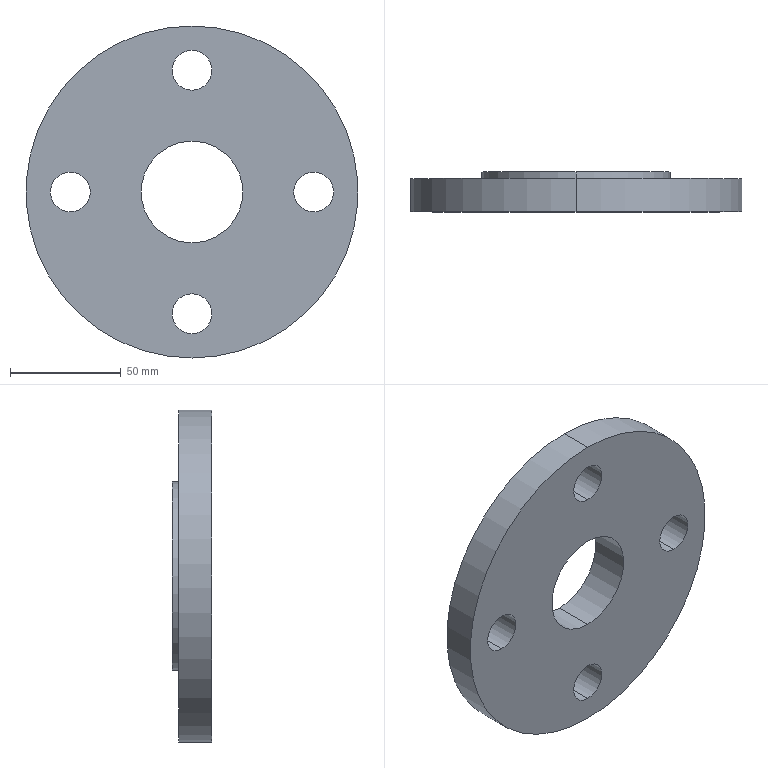Part | SolidWorks | features Extrusion 1, ICE 1 | 1 solid | 17 faces | box 150 x 18 x 150 mm | volume 236913 mm3 | cylinder 14 | plane 3 | commonest cylinder face diameters 18 x8 46 x2 85 x2 150 x2
STEP:
#1=CARTESIAN_POINT('',(0.,18.,42.5));
#2=VERTEX_POINT('',#1);
#3=CARTESIAN_POINT('',(0.,18.,-42.5));
#4=VERTEX_POINT('',#3);
#5=CARTESIAN_POINT('',(0.,18.,0.));
#6=DIRECTION('',(0.,1.,0.));
#7=DIRECTION('',(0.,0.,1.));
#8=AXIS2_PLACEMENT_3D('',#5,#6,#7);
#9=CIRCLE('',#8,42.5);
#10=EDGE_CURVE('',#2,#4,#9,.T.);
#11=ORIENTED_EDGE('',*,*,#10,.F.);
#12=CARTESIAN_POINT('',(0.,15.,42.5));
#13=VERTEX_POINT('',#12);
#14=CARTESIAN_POINT('',(0.,18.,42.5));
#15=DIRECTION('',(0.,-1.,0.));
#16=VECTOR('',#15,1000.);
#17=LINE('',#14,#16);
#18=EDGE_CURVE('',#2,#13,#17,.T.);
#19=ORIENTED_EDGE('',*,*,#18,.T.);
#20=CARTESIAN_POINT('',(0.,15.,-42.5));
#21=VERTEX_POINT('',#20);
#22=CARTESIAN_POINT('',(0.,15.,0.));
#23=DIRECTION('',(0.,1.,0.));
#24=DIRECTION('',(0.,0.,1.));
#25=AXIS2_PLACEMENT_3D('',#22,#23,#24);
#26=CIRCLE('',#25,42.5);
#27=EDGE_CURVE('',#13,#21,#26,.T.);
#28=ORIENTED_EDGE('',*,*,#27,.T.);
#29=CARTESIAN_POINT('',(0.,18.,-42.5));
#30=DIRECTION('',(0.,-1.,0.));
#31=VECTOR('',#30,1000.);
#32=LINE('',#29,#31);
#33=EDGE_CURVE('',#4,#21,#32,.T.);
#34=ORIENTED_EDGE('',*,*,#33,.F.);
#35=EDGE_LOOP('',(#11,#19,#28,#34));
#36=FACE_OUTER_BOUND('',#35,.T.);
#37=CARTESIAN_POINT('',(0.,18.,0.));
#38=DIRECTION('',(0.,-1.,0.));
#39=DIRECTION('',(0.,0.,-1.));
#40=AXIS2_PLACEMENT_3D('',#37,#38,#39);
#41=CYLINDRICAL_SURFACE('',#40,42.5);
#42=ADVANCED_FACE('',(#36),#41,.T.);
#43=CARTESIAN_POINT('',(-55.,15.,-9.));
#44=VERTEX_POINT('',#43);
#45=CARTESIAN_POINT('',(-55.,15.,9.));
#46=VERTEX_POINT('',#45);
#47=CARTESIAN_POINT('',(-55.,15.,0.));
#48=DIRECTION('',(0.,1.,0.));
#49=DIRECTION('',(0.,0.,1.));
#50=AXIS2_PLACEMENT_3D('',#47,#48,#49);
#51=CIRCLE('',#50,9.);
#52=EDGE_CURVE('',#44,#46,#51,.T.);
#53=ORIENTED_EDGE('',*,*,#52,.T.);
#54=CARTESIAN_POINT('',(-55.,0.,9.));
#55=VERTEX_POINT('',#54);
#56=CARTESIAN_POINT('',(-55.,15.,9.));
#57=DIRECTION('',(0.,-1.,0.));
#58=VECTOR('',#57,1000.);
#59=LINE('',#56,#58);
#60=EDGE_CURVE('',#46,#55,#59,.T.);
#61=ORIENTED_EDGE('',*,*,#60,.T.);
#62=CARTESIAN_POINT('',(-55.,0.,-9.));
#63=VERTEX_POINT('',#62);
#64=CARTESIAN_POINT('',(-55.,0.,0.));
#65=DIRECTION('',(0.,1.,0.));
#66=DIRECTION('',(0.,0.,1.));
#67=AXIS2_PLACEMENT_3D('',#64,#65,#66);
#68=CIRCLE('',#67,9.);
#69=EDGE_CURVE('',#63,#55,#68,.T.);
#70=ORIENTED_EDGE('',*,*,#69,.F.);
#71=CARTESIAN_POINT('',(-55.,15.,-9.));
#72=DIRECTION('',(0.,-1.,0.));
#73=VECTOR('',#72,1000.);
#74=LINE('',#71,#73);
#75=EDGE_CURVE('',#44,#63,#74,.T.);
#76=ORIENTED_EDGE('',*,*,#75,.F.);
#77=EDGE_LOOP('',(#53,#61,#70,#76));
#78=FACE_OUTER_BOUND('',#77,.T.);
#79=CARTESIAN_POINT('',(-55.,15.,0.));
#80=DIRECTION('',(0.,-1.,0.));
#81=DIRECTION('',(0.,0.,-1.));
#82=AXIS2_PLACEMENT_3D('',#79,#80,#81);
#83=CYLINDRICAL_SURFACE('',#82,9.);
#84=ADVANCED_FACE('',(#78),#83,.F.);
#85=CARTESIAN_POINT('',(0.,15.,46.));
#86=VERTEX_POINT('',#85);
#87=CARTESIAN_POINT('',(0.,15.,64.));
#88=VERTEX_POINT('',#87);
#89=CARTESIAN_POINT('',(0.,15.,55.));
#90=DIRECTION('',(0.,1.,0.));
#91=DIRECTION('',(0.,0.,1.));
#92=AXIS2_PLACEMENT_3D('',#89,#90,#91);
#93=CIRCLE('',#92,9.);
#94=EDGE_CURVE('',#86,#88,#93,.T.);
#95=ORIENTED_EDGE('',*,*,#94,.T.);
#96=CARTESIAN_POINT('',(0.,0.,64.));
#97=VERTEX_POINT('',#96);
#98=CARTESIAN_POINT('',(0.,15.,64.));
#99=DIRECTION('',(0.,-1.,0.));
#100=VECTOR('',#99,1000.);
#101=LINE('',#98,#100);
#102=EDGE_CURVE('',#88,#97,#101,.T.);
#103=ORIENTED_EDGE('',*,*,#102,.T.);
#104=CARTESIAN_POINT('',(0.,0.,46.));
#105=VERTEX_POINT('',#104);
#106=CARTESIAN_POINT('',(0.,0.,55.));
#107=DIRECTION('',(0.,1.,0.));
#108=DIRECTION('',(0.,0.,1.));
#109=AXIS2_PLACEMENT_3D('',#106,#107,#108);
#110=CIRCLE('',#109,9.);
#111=EDGE_CURVE('',#105,#97,#110,.T.);
#112=ORIENTED_EDGE('',*,*,#111,.F.);
#113=CARTESIAN_POINT('',(0.,15.,46.));
#114=DIRECTION('',(0.,-1.,0.));
#115=VECTOR('',#114,1000.);
#116=LINE('',#113,#115);
#117=EDGE_CURVE('',#86,#105,#116,.T.);
#118=ORIENTED_EDGE('',*,*,#117,.F.);
#119=EDGE_LOOP('',(#95,#103,#112,#118));
#120=FACE_OUTER_BOUND('',#119,.T.);
#121=CARTESIAN_POINT('',(0.,15.,55.));
#122=DIRECTION('',(0.,-1.,0.));
#123=DIRECTION('',(0.,0.,-1.));
#124=AXIS2_PLACEMENT_3D('',#121,#122,#123);
#125=CYLINDRICAL_SURFACE('',#124,9.);
#126=ADVANCED_FACE('',(#120),#125,.F.);
#127=CARTESIAN_POINT('',(55.,15.,-9.));
#128=VERTEX_POINT('',#127);
#129=CARTESIAN_POINT('',(55.,15.,9.));
#130=VERTEX_POINT('',#129);
#131=CARTESIAN_POINT('',(55.,15.,0.));
#132=DIRECTION('',(0.,1.,0.));
#133=DIRECTION('',(0.,0.,1.));
#134=AXIS2_PLACEMENT_3D('',#131,#132,#133);
#135=CIRCLE('',#134,9.);
#136=EDGE_CURVE('',#128,#130,#135,.T.);
#137=ORIENTED_EDGE('',*,*,#136,.T.);
#138=CARTESIAN_POINT('',(55.,0.,9.));
#139=VERTEX_POINT('',#138);
#140=CARTESIAN_POINT('',(55.,15.,9.));
#141=DIRECTION('',(0.,-1.,0.));
#142=VECTOR('',#141,1000.);
#143=LINE('',#140,#142);
#144=EDGE_CURVE('',#130,#139,#143,.T.);
#145=ORIENTED_EDGE('',*,*,#144,.T.);
#146=CARTESIAN_POINT('',(55.,0.,-9.));
#147=VERTEX_POINT('',#146);
#148=CARTESIAN_POINT('',(55.,0.,0.));
#149=DIRECTION('',(0.,1.,0.));
#150=DIRECTION('',(0.,0.,1.));
#151=AXIS2_PLACEMENT_3D('',#148,#149,#150);
#152=CIRCLE('',#151,9.);
#153=EDGE_CURVE('',#147,#139,#152,.T.);
#154=ORIENTED_EDGE('',*,*,#153,.F.);
#155=CARTESIAN_POINT('',(55.,15.,-9.));
#156=DIRECTION('',(0.,-1.,0.));
#157=VECTOR('',#156,1000.);
#158=LINE('',#155,#157);
#159=EDGE_CURVE('',#128,#147,#158,.T.);
#160=ORIENTED_EDGE('',*,*,#159,.F.);
#161=EDGE_LOOP('',(#137,#145,#154,#160));
#162=FACE_OUTER_BOUND('',#161,.T.);
#163=CARTESIAN_POINT('',(55.,15.,0.));
#164=DIRECTION('',(0.,-1.,0.));
#165=DIRECTION('',(0.,0.,-1.));
#166=AXIS2_PLACEMENT_3D('',#163,#164,#165);
#167=CYLINDRICAL_SURFACE('',#166,9.);
#168=ADVANCED_FACE('',(#162),#167,.F.);
#169=CARTESIAN_POINT('',(0.,18.,-23.));
#170=VERTEX_POINT('',#169);
#171=CARTESIAN_POINT('',(0.,18.,23.));
#172=VERTEX_POINT('',#171);
#173=CARTESIAN_POINT('',(0.,18.,0.));
#174=DIRECTION('',(0.,1.,0.));
#175=DIRECTION('',(0.,0.,1.));
#176=AXIS2_PLACEMENT_3D('',#173,#174,#175);
#177=CIRCLE('',#176,23.);
#178=EDGE_CURVE('',#170,#172,#177,.T.);
#179=ORIENTED_EDGE('',*,*,#178,.T.);
#180=CARTESIAN_POINT('',(0.,0.,23.));
#181=VERTEX_POINT('',#180);
#182=CARTESIAN_POINT('',(0.,15.,23.));
#183=DIRECTION('',(0.,-1.,0.));
#184=VECTOR('',#183,1000.);
#185=LINE('',#182,#184);
#186=EDGE_CURVE('',#172,#181,#185,.T.);
#187=ORIENTED_EDGE('',*,*,#186,.T.);
#188=CARTESIAN_POINT('',(0.,0.,-23.));
#189=VERTEX_POINT('',#188);
#190=CARTESIAN_POINT('',(0.,0.,0.));
#191=DIRECTION('',(0.,1.,0.));
#192=DIRECTION('',(0.,0.,1.));
#193=AXIS2_PLACEMENT_3D('',#190,#191,#192);
#194=CIRCLE('',#193,23.);
#195=EDGE_CURVE('',#189,#181,#194,.T.);
#196=ORIENTED_EDGE('',*,*,#195,.F.);
#197=CARTESIAN_POINT('',(0.,15.,-23.));
#198=DIRECTION('',(0.,-1.,0.));
#199=VECTOR('',#198,1000.);
#200=LINE('',#197,#199);
#201=EDGE_CURVE('',#170,#189,#200,.T.);
#202=ORIENTED_EDGE('',*,*,#201,.F.);
#203=EDGE_LOOP('',(#179,#187,#196,#202));
#204=FACE_OUTER_BOUND('',#203,.T.);
#205=CARTESIAN_POINT('',(0.,15.,0.));
#206=DIRECTION('',(0.,-1.,0.));
#207=DIRECTION('',(0.,0.,-1.));
#208=AXIS2_PLACEMENT_3D('',#205,#206,#207);
#209=CYLINDRICAL_SURFACE('',#208,23.);
#210=ADVANCED_FACE('',(#204),#209,.F.);
#211=CARTESIAN_POINT('',(0.,15.,-64.));
#212=VERTEX_POINT('',#211);
#213=CARTESIAN_POINT('',(0.,15.,-46.));
#214=VERTEX_POINT('',#213);
#215=CARTESIAN_POINT('',(0.,15.,-55.));
#216=DIRECTION('',(0.,1.,0.));
#217=DIRECTION('',(0.,0.,1.));
#218=AXIS2_PLACEMENT_3D('',#215,#216,#217);
#219=CIRCLE('',#218,9.);
#220=EDGE_CURVE('',#212,#214,#219,.T.);
#221=ORIENTED_EDGE('',*,*,#220,.T.);
#222=CARTESIAN_POINT('',(0.,0.,-46.));
#223=VERTEX_POINT('',#222);
#224=CARTESIAN_POINT('',(0.,15.,-46.));
#225=DIRECTION('',(0.,-1.,0.));
#226=VECTOR('',#225,1000.);
#227=LINE('',#224,#226);
#228=EDGE_CURVE('',#214,#223,#227,.T.);
#229=ORIENTED_EDGE('',*,*,#228,.T.);
#230=CARTESIAN_POINT('',(0.,0.,-64.));
#231=VERTEX_POINT('',#230);
#232=CARTESIAN_POINT('',(0.,0.,-55.));
#233=DIRECTION('',(0.,1.,0.));
#234=DIRECTION('',(0.,0.,1.));
#235=AXIS2_PLACEMENT_3D('',#232,#233,#234);
#236=CIRCLE('',#235,9.);
#237=EDGE_CURVE('',#231,#223,#236,.T.);
#238=ORIENTED_EDGE('',*,*,#237,.F.);
#239=CARTESIAN_POINT('',(0.,15.,-64.));
#240=DIRECTION('',(0.,-1.,0.));
#241=VECTOR('',#240,1000.);
#242=LINE('',#239,#241);
#243=EDGE_CURVE('',#212,#231,#242,.T.);
#244=ORIENTED_EDGE('',*,*,#243,.F.);
#245=EDGE_LOOP('',(#221,#229,#238,#244));
#246=FACE_OUTER_BOUND('',#245,.T.);
#247=CARTESIAN_POINT('',(0.,15.,-55.));
#248=DIRECTION('',(0.,-1.,0.));
#249=DIRECTION('',(0.,0.,-1.));
#250=AXIS2_PLACEMENT_3D('',#247,#248,#249);
#251=CYLINDRICAL_SURFACE('',#250,9.);
#252=ADVANCED_FACE('',(#246),#251,.F.);
#253=CARTESIAN_POINT('',(0.,15.,75.));
#254=VERTEX_POINT('',#253);
#255=CARTESIAN_POINT('',(0.,15.,-75.));
#256=VERTEX_POINT('',#255);
#257=CARTESIAN_POINT('',(0.,15.,0.));
#258=DIRECTION('',(0.,1.,0.));
#259=DIRECTION('',(0.,0.,1.));
#260=AXIS2_PLACEMENT_3D('',#257,#258,#259);
#261=CIRCLE('',#260,75.);
#262=EDGE_CURVE('',#254,#256,#261,.T.);
#263=ORIENTED_EDGE('',*,*,#262,.F.);
#264=CARTESIAN_POINT('',(0.,0.,75.));
#265=VERTEX_POINT('',#264);
#266=CARTESIAN_POINT('',(0.,15.,75.));
#267=DIRECTION('',(0.,-1.,0.));
#268=VECTOR('',#267,1000.);
#269=LINE('',#266,#268);
#270=EDGE_CURVE('',#254,#265,#269,.T.);
#271=ORIENTED_EDGE('',*,*,#270,.T.);
#272=CARTESIAN_POINT('',(0.,0.,-75.));
#273=VERTEX_POINT('',#272);
#274=CARTESIAN_POINT('',(0.,0.,0.));
#275=DIRECTION('',(0.,1.,0.));
#276=DIRECTION('',(0.,0.,1.));
#277=AXIS2_PLACEMENT_3D('',#274,#275,#276);
#278=CIRCLE('',#277,75.);
#279=EDGE_CURVE('',#265,#273,#278,.T.);
#280=ORIENTED_EDGE('',*,*,#279,.T.);
#281=CARTESIAN_POINT('',(0.,15.,-75.));
#282=DIRECTION('',(0.,-1.,0.));
#283=VECTOR('',#282,1000.);
#284=LINE('',#281,#283);
#285=EDGE_CURVE('',#256,#273,#284,.T.);
#286=ORIENTED_EDGE('',*,*,#285,.F.);
#287=EDGE_LOOP('',(#263,#271,#280,#286));
#288=FACE_OUTER_BOUND('',#287,.T.);
#289=CARTESIAN_POINT('',(0.,15.,0.));
#290=DIRECTION('',(0.,-1.,0.));
#291=DIRECTION('',(0.,0.,-1.));
#292=AXIS2_PLACEMENT_3D('',#289,#290,#291);
#293=CYLINDRICAL_SURFACE('',#292,75.);
#294=ADVANCED_FACE('',(#288),#293,.T.);
#295=CARTESIAN_POINT('',(0.,15.,0.));
#296=DIRECTION('',(0.,1.,0.));
#297=DIRECTION('',(0.,0.,1.));
#298=AXIS2_PLACEMENT_3D('',#295,#296,#297);
#299=CIRCLE('',#298,42.5);
#300=EDGE_CURVE('',#21,#13,#299,.T.);
#301=ORIENTED_EDGE('',*,*,#300,.F.);
#302=ORIENTED_EDGE('',*,*,#27,.F.);
#303=EDGE_LOOP('',(#301,#302));
#304=FACE_BOUND('',#303,.T.);
#305=ORIENTED_EDGE('',*,*,#94,.F.);
#306=CARTESIAN_POINT('',(0.,15.,55.));
#307=DIRECTION('',(0.,1.,0.));
#308=DIRECTION('',(0.,0.,1.));
#309=AXIS2_PLACEMENT_3D('',#306,#307,#308);
#310=CIRCLE('',#309,9.);
#311=EDGE_CURVE('',#88,#86,#310,.T.);
#312=ORIENTED_EDGE('',*,*,#311,.F.);
#313=EDGE_LOOP('',(#305,#312));
#314=FACE_BOUND('',#313,.T.);
#315=CARTESIAN_POINT('',(0.,15.,0.));
#316=DIRECTION('',(0.,1.,0.));
#317=DIRECTION('',(0.,0.,1.));
#318=AXIS2_PLACEMENT_3D('',#315,#316,#317);
#319=CIRCLE('',#318,75.);
#320=EDGE_CURVE('',#256,#254,#319,.T.);
#321=ORIENTED_EDGE('',*,*,#320,.T.);
#322=ORIENTED_EDGE('',*,*,#262,.T.);
#323=EDGE_LOOP('',(#321,#322));
#324=FACE_OUTER_BOUND('',#323,.T.);
#325=ORIENTED_EDGE('',*,*,#220,.F.);
#326=CARTESIAN_POINT('',(0.,15.,-55.));
#327=DIRECTION('',(0.,1.,0.));
#328=DIRECTION('',(0.,0.,1.));
#329=AXIS2_PLACEMENT_3D('',#326,#327,#328);
#330=CIRCLE('',#329,9.);
#331=EDGE_CURVE('',#214,#212,#330,.T.);
#332=ORIENTED_EDGE('',*,*,#331,.F.);
#333=EDGE_LOOP('',(#325,#332));
#334=FACE_BOUND('',#333,.T.);
#335=ORIENTED_EDGE('',*,*,#136,.F.);
#336=CARTESIAN_POINT('',(55.,15.,0.));
#337=DIRECTION('',(0.,1.,0.));
#338=DIRECTION('',(0.,0.,1.));
#339=AXIS2_PLACEMENT_3D('',#336,#337,#338);
#340=CIRCLE('',#339,9.);
#341=EDGE_CURVE('',#130,#128,#340,.T.);
#342=ORIENTED_EDGE('',*,*,#341,.F.);
#343=EDGE_LOOP('',(#335,#342));
#344=FACE_BOUND('',#343,.T.);
#345=ORIENTED_EDGE('',*,*,#52,.F.);
#346=CARTESIAN_POINT('',(-55.,15.,0.));
#347=DIRECTION('',(0.,1.,0.));
#348=DIRECTION('',(0.,0.,1.));
#349=AXIS2_PLACEMENT_3D('',#346,#347,#348);
#350=CIRCLE('',#349,9.);
#351=EDGE_CURVE('',#46,#44,#350,.T.);
#352=ORIENTED_EDGE('',*,*,#351,.F.);
#353=EDGE_LOOP('',(#345,#352));
#354=FACE_BOUND('',#353,.T.);
#355=CARTESIAN_POINT('',(0.,15.,0.));
#356=DIRECTION('',(0.,1.,0.));
#357=DIRECTION('',(0.,0.,1.));
#358=AXIS2_PLACEMENT_3D('',#355,#356,#357);
#359=PLANE('',#358);
#360=ADVANCED_FACE('',(#304,#314,#324,#334,#344,#354),#359,.T.);
#361=CARTESIAN_POINT('',(0.,0.,0.));
#362=DIRECTION('',(0.,1.,0.));
#363=DIRECTION('',(0.,0.,1.));
#364=AXIS2_PLACEMENT_3D('',#361,#362,#363);
#365=CIRCLE('',#364,75.);
#366=EDGE_CURVE('',#273,#265,#365,.T.);
#367=ORIENTED_EDGE('',*,*,#366,.F.);
#368=ORIENTED_EDGE('',*,*,#279,.F.);
#369=EDGE_LOOP('',(#367,#368));
#370=FACE_OUTER_BOUND('',#369,.T.);
#371=ORIENTED_EDGE('',*,*,#237,.T.);
#372=CARTESIAN_POINT('',(0.,0.,-55.));
#373=DIRECTION('',(0.,1.,0.));
#374=DIRECTION('',(0.,0.,1.));
#375=AXIS2_PLACEMENT_3D('',#372,#373,#374);
#376=CIRCLE('',#375,9.);
#377=EDGE_CURVE('',#223,#231,#376,.T.);
#378=ORIENTED_EDGE('',*,*,#377,.T.);
#379=EDGE_LOOP('',(#371,#378));
#380=FACE_BOUND('',#379,.T.);
#381=ORIENTED_EDGE('',*,*,#195,.T.);
#382=CARTESIAN_POINT('',(0.,0.,0.));
#383=DIRECTION('',(0.,1.,0.));
#384=DIRECTION('',(0.,0.,1.));
#385=AXIS2_PLACEMENT_3D('',#382,#383,#384);
#386=CIRCLE('',#385,23.);
#387=EDGE_CURVE('',#181,#189,#386,.T.);
#388=ORIENTED_EDGE('',*,*,#387,.T.);
#389=EDGE_LOOP('',(#381,#388));
#390=FACE_BOUND('',#389,.T.);
#391=ORIENTED_EDGE('',*,*,#153,.T.);
#392=CARTESIAN_POINT('',(55.,0.,0.));
#393=DIRECTION('',(0.,1.,0.));
#394=DIRECTION('',(0.,0.,1.));
#395=AXIS2_PLACEMENT_3D('',#392,#393,#394);
#396=CIRCLE('',#395,9.);
#397=EDGE_CURVE('',#139,#147,#396,.T.);
#398=ORIENTED_EDGE('',*,*,#397,.T.);
#399=EDGE_LOOP('',(#391,#398));
#400=FACE_BOUND('',#399,.T.);
#401=ORIENTED_EDGE('',*,*,#111,.T.);
#402=CARTESIAN_POINT('',(0.,0.,55.));
#403=DIRECTION('',(0.,1.,0.));
#404=DIRECTION('',(0.,0.,1.));
#405=AXIS2_PLACEMENT_3D('',#402,#403,#404);
#406=CIRCLE('',#405,9.);
#407=EDGE_CURVE('',#97,#105,#406,.T.);
#408=ORIENTED_EDGE('',*,*,#407,.T.);
#409=EDGE_LOOP('',(#401,#408));
#410=FACE_BOUND('',#409,.T.);
#411=ORIENTED_EDGE('',*,*,#69,.T.);
#412=CARTESIAN_POINT('',(-55.,0.,0.));
#413=DIRECTION('',(0.,1.,0.));
#414=DIRECTION('',(0.,0.,1.));
#415=AXIS2_PLACEMENT_3D('',#412,#413,#414);
#416=CIRCLE('',#415,9.);
#417=EDGE_CURVE('',#55,#63,#416,.T.);
#418=ORIENTED_EDGE('',*,*,#417,.T.);
#419=EDGE_LOOP('',(#411,#418));
#420=FACE_BOUND('',#419,.T.);
#421=CARTESIAN_POINT('',(0.,0.,0.));
#422=DIRECTION('',(0.,1.,0.));
#423=DIRECTION('',(0.,0.,1.));
#424=AXIS2_PLACEMENT_3D('',#421,#422,#423);
#425=PLANE('',#424);
#426=ADVANCED_FACE('',(#370,#380,#390,#400,#410,#420),#425,.F.);
#427=ORIENTED_EDGE('',*,*,#270,.F.);
#428=ORIENTED_EDGE('',*,*,#320,.F.);
#429=ORIENTED_EDGE('',*,*,#285,.T.);
#430=ORIENTED_EDGE('',*,*,#366,.T.);
#431=EDGE_LOOP('',(#427,#428,#429,#430));
#432=FACE_OUTER_BOUND('',#431,.T.);
#433=CARTESIAN_POINT('',(0.,15.,0.));
#434=DIRECTION('',(0.,-1.,0.));
#435=DIRECTION('',(0.,0.,-1.));
#436=AXIS2_PLACEMENT_3D('',#433,#434,#435);
#437=CYLINDRICAL_SURFACE('',#436,75.);
#438=ADVANCED_FACE('',(#432),#437,.T.);
#439=ORIENTED_EDGE('',*,*,#228,.F.);
#440=ORIENTED_EDGE('',*,*,#331,.T.);
#441=ORIENTED_EDGE('',*,*,#243,.T.);
#442=ORIENTED_EDGE('',*,*,#377,.F.);
#443=EDGE_LOOP('',(#439,#440,#441,#442));
#444=FACE_OUTER_BOUND('',#443,.T.);
#445=CARTESIAN_POINT('',(0.,15.,-55.));
#446=DIRECTION('',(0.,-1.,0.));
#447=DIRECTION('',(0.,0.,-1.));
#448=AXIS2_PLACEMENT_3D('',#445,#446,#447);
#449=CYLINDRICAL_SURFACE('',#448,9.);
#450=ADVANCED_FACE('',(#444),#449,.F.);
#451=ORIENTED_EDGE('',*,*,#186,.F.);
#452=CARTESIAN_POINT('',(0.,18.,0.));
#453=DIRECTION('',(0.,1.,0.));
#454=DIRECTION('',(0.,0.,1.));
#455=AXIS2_PLACEMENT_3D('',#452,#453,#454);
#456=CIRCLE('',#455,23.);
#457=EDGE_CURVE('',#172,#170,#456,.T.);
#458=ORIENTED_EDGE('',*,*,#457,.T.);
#459=ORIENTED_EDGE('',*,*,#201,.T.);
#460=ORIENTED_EDGE('',*,*,#387,.F.);
#461=EDGE_LOOP('',(#451,#458,#459,#460));
#462=FACE_OUTER_BOUND('',#461,.T.);
#463=CARTESIAN_POINT('',(0.,15.,0.));
#464=DIRECTION('',(0.,-1.,0.));
#465=DIRECTION('',(0.,0.,-1.));
#466=AXIS2_PLACEMENT_3D('',#463,#464,#465);
#467=CYLINDRICAL_SURFACE('',#466,23.);
#468=ADVANCED_FACE('',(#462),#467,.F.);
#469=ORIENTED_EDGE('',*,*,#144,.F.);
#470=ORIENTED_EDGE('',*,*,#341,.T.);
#471=ORIENTED_EDGE('',*,*,#159,.T.);
#472=ORIENTED_EDGE('',*,*,#397,.F.);
#473=EDGE_LOOP('',(#469,#470,#471,#472));
#474=FACE_OUTER_BOUND('',#473,.T.);
#475=CARTESIAN_POINT('',(55.,15.,0.));
#476=DIRECTION('',(0.,-1.,0.));
#477=DIRECTION('',(0.,0.,-1.));
#478=AXIS2_PLACEMENT_3D('',#475,#476,#477);
#479=CYLINDRICAL_SURFACE('',#478,9.);
#480=ADVANCED_FACE('',(#474),#479,.F.);
#481=ORIENTED_EDGE('',*,*,#102,.F.);
#482=ORIENTED_EDGE('',*,*,#311,.T.);
#483=ORIENTED_EDGE('',*,*,#117,.T.);
#484=ORIENTED_EDGE('',*,*,#407,.F.);
#485=EDGE_LOOP('',(#481,#482,#483,#484));
#486=FACE_OUTER_BOUND('',#485,.T.);
#487=CARTESIAN_POINT('',(0.,15.,55.));
#488=DIRECTION('',(0.,-1.,0.));
#489=DIRECTION('',(0.,0.,-1.));
#490=AXIS2_PLACEMENT_3D('',#487,#488,#489);
#491=CYLINDRICAL_SURFACE('',#490,9.);
#492=ADVANCED_FACE('',(#486),#491,.F.);
#493=ORIENTED_EDGE('',*,*,#60,.F.);
#494=ORIENTED_EDGE('',*,*,#351,.T.);
#495=ORIENTED_EDGE('',*,*,#75,.T.);
#496=ORIENTED_EDGE('',*,*,#417,.F.);
#497=EDGE_LOOP('',(#493,#494,#495,#496));
#498=FACE_OUTER_BOUND('',#497,.T.);
#499=CARTESIAN_POINT('',(-55.,15.,0.));
#500=DIRECTION('',(0.,-1.,0.));
#501=DIRECTION('',(0.,0.,-1.));
#502=AXIS2_PLACEMENT_3D('',#499,#500,#501);
#503=CYLINDRICAL_SURFACE('',#502,9.);
#504=ADVANCED_FACE('',(#498),#503,.F.);
#505=CARTESIAN_POINT('',(0.,18.,0.));
#506=DIRECTION('',(0.,1.,0.));
#507=DIRECTION('',(0.,0.,1.));
#508=AXIS2_PLACEMENT_3D('',#505,#506,#507);
#509=CIRCLE('',#508,42.5);
#510=EDGE_CURVE('',#4,#2,#509,.T.);
#511=ORIENTED_EDGE('',*,*,#510,.T.);
#512=ORIENTED_EDGE('',*,*,#10,.T.);
#513=EDGE_LOOP('',(#511,#512));
#514=FACE_OUTER_BOUND('',#513,.T.);
#515=ORIENTED_EDGE('',*,*,#178,.F.);
#516=ORIENTED_EDGE('',*,*,#457,.F.);
#517=EDGE_LOOP('',(#515,#516));
#518=FACE_BOUND('',#517,.T.);
#519=CARTESIAN_POINT('',(0.,18.,0.));
#520=DIRECTION('',(0.,1.,0.));
#521=DIRECTION('',(0.,0.,1.));
#522=AXIS2_PLACEMENT_3D('',#519,#520,#521);
#523=PLANE('',#522);
#524=ADVANCED_FACE('',(#514,#518),#523,.T.);
#525=ORIENTED_EDGE('',*,*,#18,.F.);
#526=ORIENTED_EDGE('',*,*,#510,.F.);
#527=ORIENTED_EDGE('',*,*,#33,.T.);
#528=ORIENTED_EDGE('',*,*,#300,.T.);
#529=EDGE_LOOP('',(#525,#526,#527,#528));
#530=FACE_OUTER_BOUND('',#529,.T.);
#531=CARTESIAN_POINT('',(0.,18.,0.));
#532=DIRECTION('',(0.,-1.,0.));
#533=DIRECTION('',(0.,0.,-1.));
#534=AXIS2_PLACEMENT_3D('',#531,#532,#533);
#535=CYLINDRICAL_SURFACE('',#534,42.5);
#536=ADVANCED_FACE('',(#530),#535,.T.);
#537=CLOSED_SHELL('',(#42,#84,#126,#168,#210,#252,#294,#360,#426,#438,#450,#468,#480,#492,#504,#524,#536));
#538=MANIFOLD_SOLID_BREP('',#537);
#539=CARTESIAN_POINT('',(0.,0.,0.));
#540=DIRECTION('',(0.,0.,1.));
#541=DIRECTION('',(1.,0.,0.));
#542=AXIS2_PLACEMENT_3D('',#539,#540,#541);
#543=(LENGTH_UNIT()NAMED_UNIT(*)SI_UNIT(.MILLI.,.METRE.));
#544=UNCERTAINTY_MEASURE_WITH_UNIT(LENGTH_MEASURE(0.00001),#543,'','');
#545=(NAMED_UNIT(*)PLANE_ANGLE_UNIT()SI_UNIT($,.RADIAN.));
#546=(NAMED_UNIT(*)SI_UNIT($,.STERADIAN.)SOLID_ANGLE_UNIT());
#547=(GEOMETRIC_REPRESENTATION_CONTEXT(3)GLOBAL_UNCERTAINTY_ASSIGNED_CONTEXT((#544))GLOBAL_UNIT_ASSIGNED_CONTEXT((#543,#545,#546))REPRESENTATION_CONTEXT('',''));
#548=ADVANCED_BREP_SHAPE_REPRESENTATION('',(#538,#542),#547);